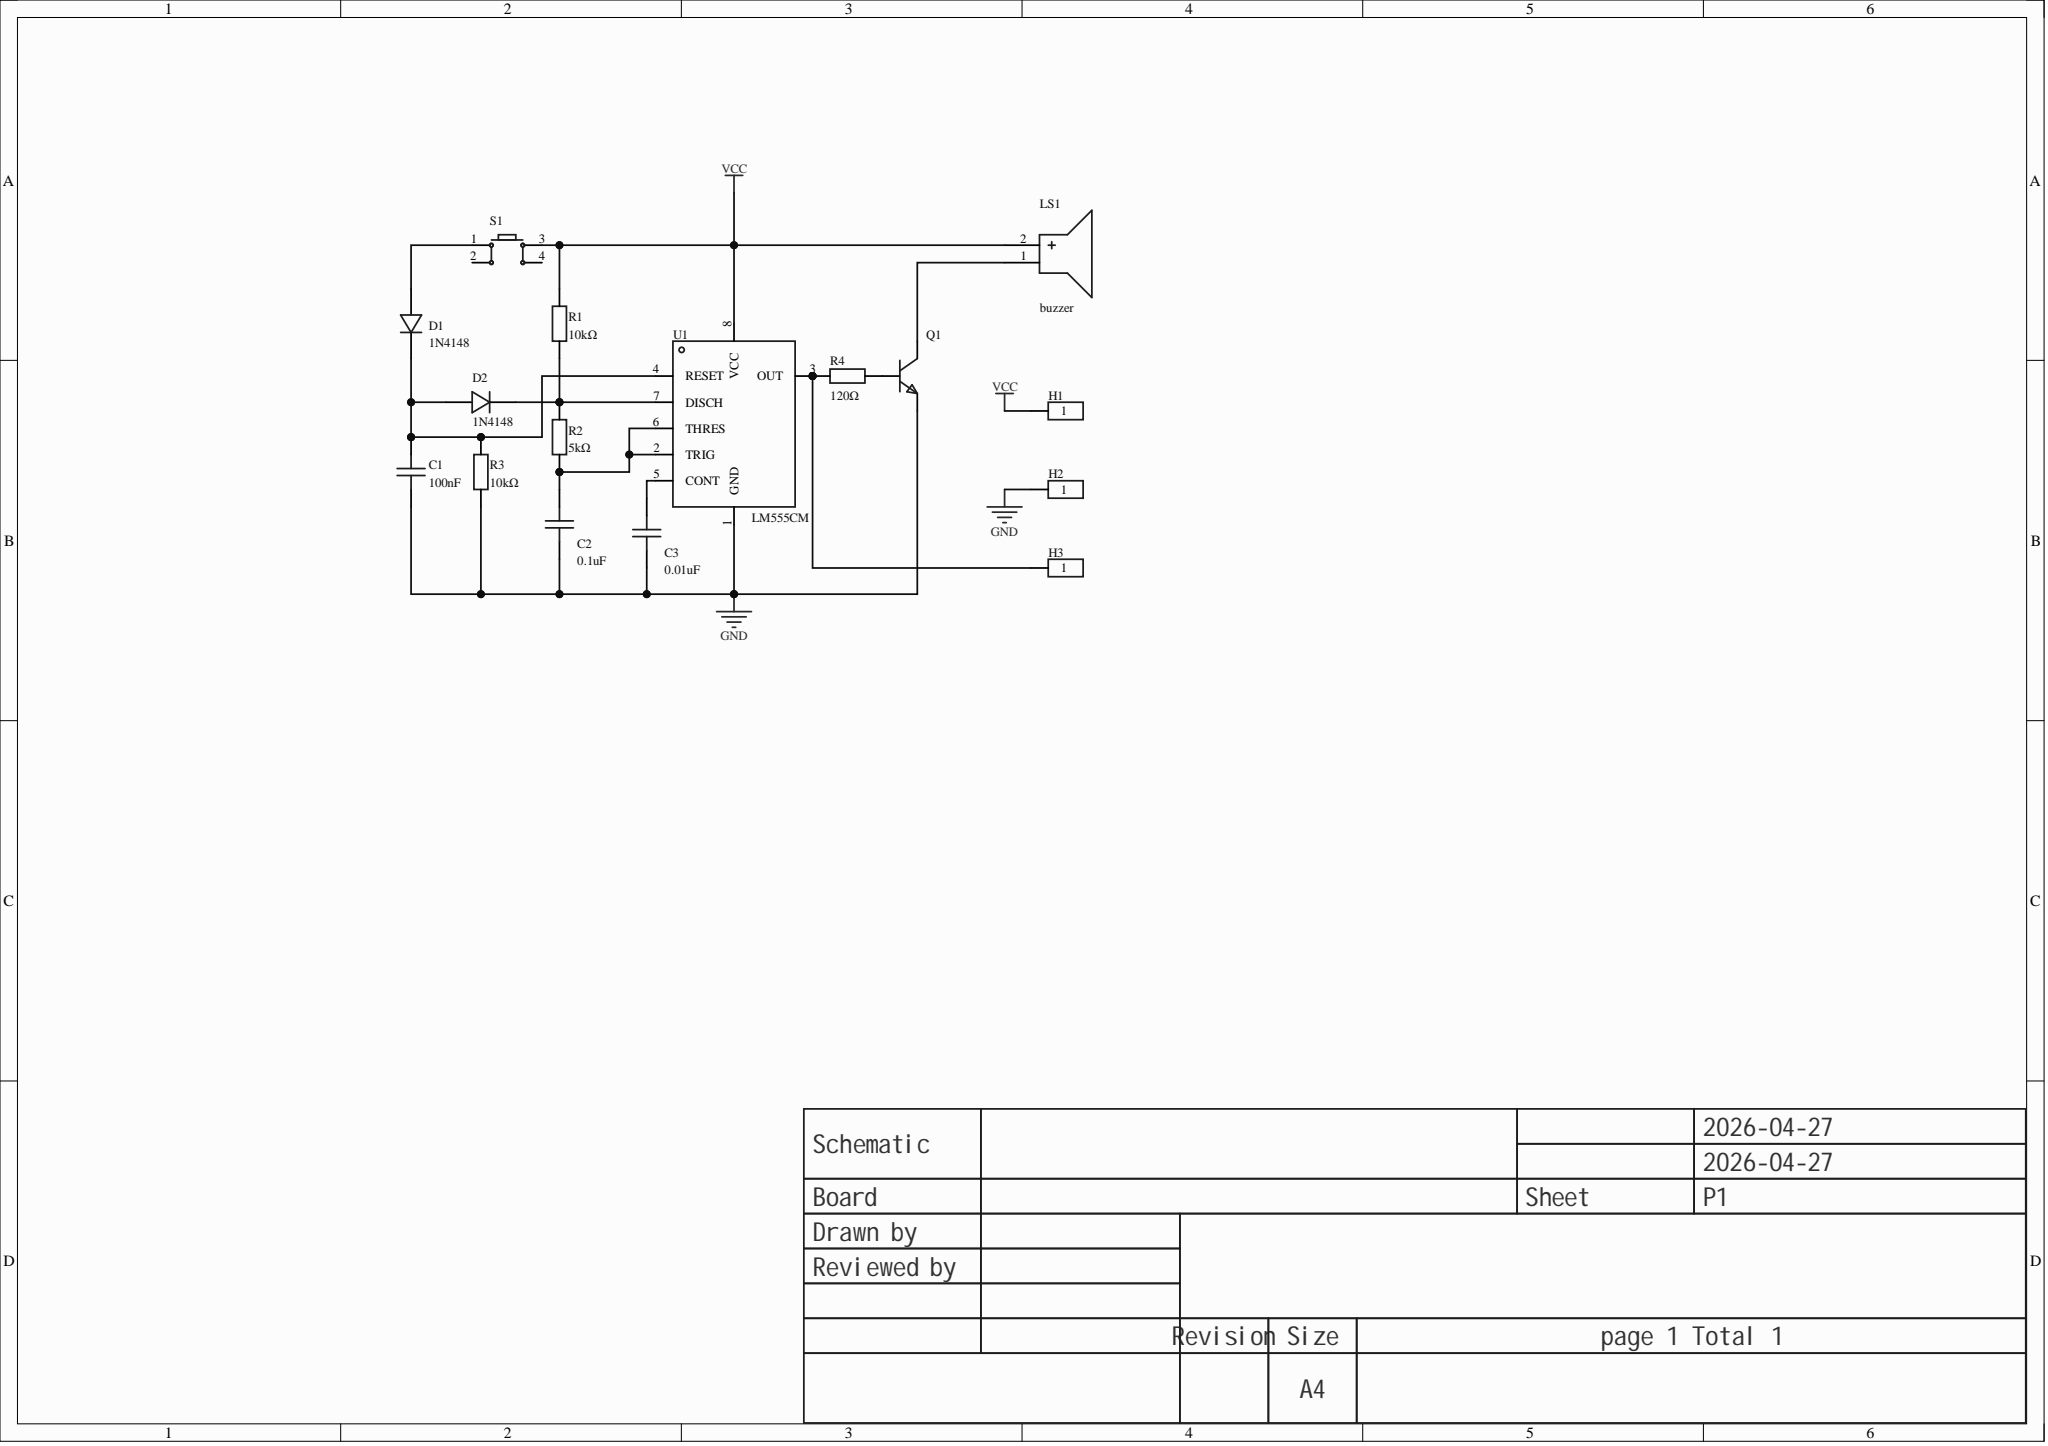Circuit board | Altium Designer | 16 parts | 10 nets
Bill of materials:
Comment,Description,Designator,Footprint,LibRef,Quantity
"100nF","","C1","CAP-TH_L5.0-W2.5-P5.00-D1.0","100nF","1"
"0.1uF","","C2","CAP-TH_L5.0-W2.5-P5.00-D1.0","100nF","1"
"0.01uF","","C3","CAP-TH_L5.0-W2.5-P5.00-D1.0","100nF","1"
"1N4148","","D1, D2","DO-35_BD2.2-L4.0-D0.50_1N4148","1N4148_C9900036548","2"
"","","H1, H2, H3","HDR-TH_1P-V-M_XKB_X4611WV-01I-C28D40","HDR-M_2.54_1x1P","3"
"buzzer","","LS1","BUZ-TH_BD12.0-P6.00-D0.9-RD","buzzer","1"
"","","Q1","S8050_TO_92","S8050_TO_NPN","1"
"10kΩ","","R1, R3","Res_1/8W","Res_AXIAL-1/8W","2"
"5kΩ","","R2","Res_1/8W","Res_AXIAL-1/8W","1"
"120Ω","","R4","Res_1/8W","Res_AXIAL-1/8W","1"
"","","S1","SW-TH_4P-L6.0-W6.0-P4.50-LS6.5","Key_TH_6x6x6","1"
"LM555CM","NE555 single-precision timer","U1","PDIP-8_L9.6-W6.4-P2.54-LS7.9-BL-1","NE555PE4","1"
Netlist (Protel format):
[
C1
CAP-TH_L5.0-W2.5-P5.00-D1.0
100nF



]
[
C2
CAP-TH_L5.0-W2.5-P5.00-D1.0
0.1uF



]
[
C3
CAP-TH_L5.0-W2.5-P5.00-D1.0
0.01uF



]
[
D1
DO-35_BD2.2-L4.0-D0.50_1N4148
1N4148



]
[
D2
DO-35_BD2.2-L4.0-D0.50_1N4148
1N4148



]
[
H1
HDR-TH_1P-V-M_XKB_X4611WV-01I-C28D40




]
[
H2
HDR-TH_1P-V-M_XKB_X4611WV-01I-C28D40




]
[
H3
HDR-TH_1P-V-M_XKB_X4611WV-01I-C28D40




]
[
LS1
BUZ-TH_BD12.0-P6.00-D0.9-RD
buzzer



]
[
Q1
S8050_TO_92




]
[
R1
Res_1/8W
10kΩ



]
[
R2
Res_1/8W
5kΩ



]
[
R3
Res_1/8W
10kΩ



]
[
R4
Res_1/8W
120Ω



]
[
S1
SW-TH_4P-L6.0-W6.0-P4.50-LS6.5




]
[
U1
PDIP-8_L9.6-W6.4-P2.54-LS7.9-BL-1
LM555CM



]
(
VCC
H1-1
LS1-2
R1-2
S1-3
U1-8
)
(
NetQ1_2
Q1-2
R4-2
)
(
NetLS1_1
LS1-1
Q1-3
)
(
NetH3_1
H3-1
R4-1
U1-3
)
(
NetD2_2
D2-2
R1-1
R2-2
U1-7
)
(
NetD1_1
D1-1
S1-1
)
(
NetC3_1
C3-1
U1-5
)
(
NetC2_1
C2-1
R2-1
U1-2
U1-6
)
(
NetC1_1
C1-1
D1-2
D2-1
R3-2
U1-4
)
(
GND
C1-2
C2-2
C3-2
H2-1
Q1-1
R3-1
U1-1
)